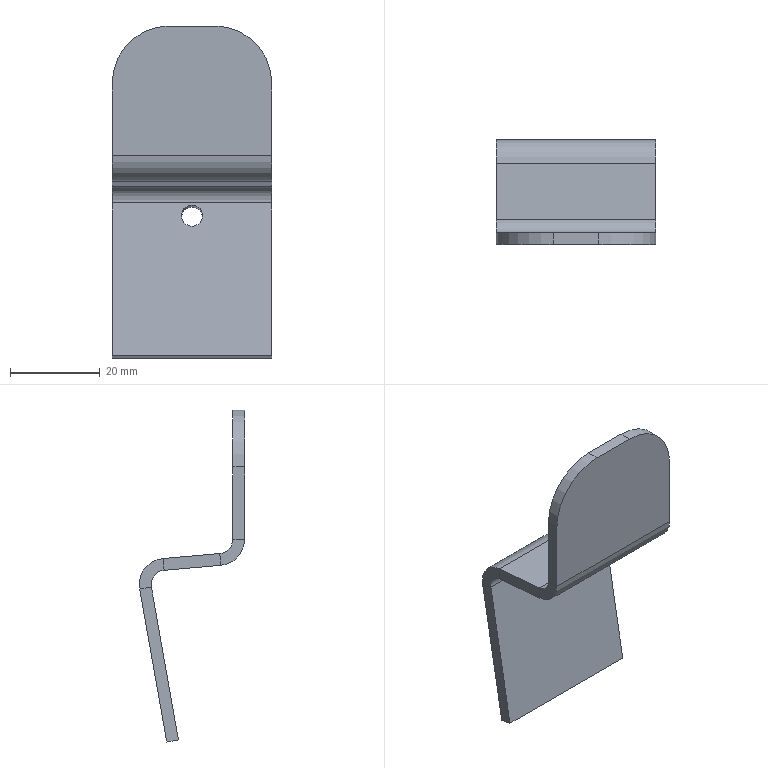Part | NX | features BREP 1 | 1 solid | 26 faces | box 35.56 x 23.477 x 74.022 mm | volume 8250 mm3 | plane 18 | cylinder 8 | commonest cylinder face diameters 4.775 x2 6.35 x2 11.633 x2 25.4 x2
STEP:
#1=CARTESIAN_POINT('',(17.78,0.,-12.7));
#2=VERTEX_POINT('',#1);
#3=CARTESIAN_POINT('',(17.78,0.,-28.841));
#4=VERTEX_POINT('',#3);
#5=CARTESIAN_POINT('',(17.78,0.,-12.7));
#6=DIRECTION('',(0.,0.,-1.));
#7=VECTOR('',#6,1000.);
#8=LINE('',#5,#7);
#9=EDGE_CURVE('',#2,#4,#8,.T.);
#10=ORIENTED_EDGE('',*,*,#9,.T.);
#11=CARTESIAN_POINT('',(-17.78,0.,-28.841));
#12=VERTEX_POINT('',#11);
#13=CARTESIAN_POINT('',(-17.78,0.,-28.841));
#14=DIRECTION('',(1.,0.,0.));
#15=VECTOR('',#14,1000.);
#16=LINE('',#13,#15);
#17=EDGE_CURVE('',#12,#4,#16,.T.);
#18=ORIENTED_EDGE('',*,*,#17,.F.);
#19=CARTESIAN_POINT('',(-17.78,0.,-12.7));
#20=VERTEX_POINT('',#19);
#21=CARTESIAN_POINT('',(-17.78,0.,-28.841));
#22=DIRECTION('',(0.,0.,1.));
#23=VECTOR('',#22,1000.);
#24=LINE('',#21,#23);
#25=EDGE_CURVE('',#12,#20,#24,.T.);
#26=ORIENTED_EDGE('',*,*,#25,.T.);
#27=CARTESIAN_POINT('',(-5.08,0.,0.));
#28=VERTEX_POINT('',#27);
#29=CARTESIAN_POINT('',(-5.08,0.,-12.7));
#30=DIRECTION('',(0.,1.,0.));
#31=DIRECTION('',(-1.,0.,0.));
#32=AXIS2_PLACEMENT_3D('',#29,#30,#31);
#33=CIRCLE('',#32,12.7);
#34=EDGE_CURVE('',#20,#28,#33,.T.);
#35=ORIENTED_EDGE('',*,*,#34,.T.);
#36=CARTESIAN_POINT('',(5.08,0.,0.));
#37=VERTEX_POINT('',#36);
#38=CARTESIAN_POINT('',(-5.08,0.,0.));
#39=DIRECTION('',(1.,0.,0.));
#40=VECTOR('',#39,1000.);
#41=LINE('',#38,#40);
#42=EDGE_CURVE('',#28,#37,#41,.T.);
#43=ORIENTED_EDGE('',*,*,#42,.T.);
#44=CARTESIAN_POINT('',(5.08,0.,-12.7));
#45=DIRECTION('',(0.,1.,0.));
#46=DIRECTION('',(0.,0.,1.));
#47=AXIS2_PLACEMENT_3D('',#44,#45,#46);
#48=CIRCLE('',#47,12.7);
#49=EDGE_CURVE('',#37,#2,#48,.T.);
#50=ORIENTED_EDGE('',*,*,#49,.T.);
#51=EDGE_LOOP('',(#10,#18,#26,#35,#43,#50));
#52=FACE_BOUND('',#51,.T.);
#53=CARTESIAN_POINT('',(0.,0.,0.));
#54=DIRECTION('',(0.,1.,0.));
#55=DIRECTION('',(1.,0.,0.));
#56=AXIS2_PLACEMENT_3D('',#53,#54,#55);
#57=PLANE('',#56);
#58=ADVANCED_FACE('',(#52),#57,.T.);
#59=CARTESIAN_POINT('',(17.78,-2.642,-12.7));
#60=VERTEX_POINT('',#59);
#61=CARTESIAN_POINT('',(5.08,-2.642,0.));
#62=VERTEX_POINT('',#61);
#63=CARTESIAN_POINT('',(5.08,-2.642,-12.7));
#64=DIRECTION('',(0.,-1.,0.));
#65=DIRECTION('',(1.,0.,0.));
#66=AXIS2_PLACEMENT_3D('',#63,#64,#65);
#67=CIRCLE('',#66,12.7);
#68=EDGE_CURVE('',#60,#62,#67,.T.);
#69=ORIENTED_EDGE('',*,*,#68,.F.);
#70=CARTESIAN_POINT('',(17.78,-2.642,-12.7));
#71=DIRECTION('',(0.,1.,0.));
#72=VECTOR('',#71,1000.);
#73=LINE('',#70,#72);
#74=EDGE_CURVE('',#60,#2,#73,.T.);
#75=ORIENTED_EDGE('',*,*,#74,.T.);
#76=ORIENTED_EDGE('',*,*,#49,.F.);
#77=CARTESIAN_POINT('',(5.08,-2.642,0.));
#78=DIRECTION('',(0.,1.,0.));
#79=VECTOR('',#78,1000.);
#80=LINE('',#77,#79);
#81=EDGE_CURVE('',#62,#37,#80,.T.);
#82=ORIENTED_EDGE('',*,*,#81,.F.);
#83=EDGE_LOOP('',(#69,#75,#76,#82));
#84=FACE_BOUND('',#83,.T.);
#85=CARTESIAN_POINT('',(5.08,-2.756,-12.7));
#86=DIRECTION('',(0.,1.,0.));
#87=DIRECTION('',(0.,0.,1.));
#88=AXIS2_PLACEMENT_3D('',#85,#86,#87);
#89=CYLINDRICAL_SURFACE('',#88,12.7);
#90=ADVANCED_FACE('',(#84),#89,.T.);
#91=ORIENTED_EDGE('',*,*,#42,.F.);
#92=CARTESIAN_POINT('',(-5.08,-2.642,0.));
#93=VERTEX_POINT('',#92);
#94=CARTESIAN_POINT('',(-5.08,-2.642,0.));
#95=DIRECTION('',(0.,1.,0.));
#96=VECTOR('',#95,1000.);
#97=LINE('',#94,#96);
#98=EDGE_CURVE('',#93,#28,#97,.T.);
#99=ORIENTED_EDGE('',*,*,#98,.F.);
#100=CARTESIAN_POINT('',(-5.08,-2.642,0.));
#101=DIRECTION('',(1.,0.,0.));
#102=VECTOR('',#101,1000.);
#103=LINE('',#100,#102);
#104=EDGE_CURVE('',#93,#62,#103,.T.);
#105=ORIENTED_EDGE('',*,*,#104,.T.);
#106=ORIENTED_EDGE('',*,*,#81,.T.);
#107=EDGE_LOOP('',(#91,#99,#105,#106));
#108=FACE_BOUND('',#107,.T.);
#109=CARTESIAN_POINT('',(0.,-1.321,0.));
#110=DIRECTION('',(0.,0.,1.));
#111=DIRECTION('',(1.,0.,0.));
#112=AXIS2_PLACEMENT_3D('',#109,#110,#111);
#113=PLANE('',#112);
#114=ADVANCED_FACE('',(#108),#113,.T.);
#115=ORIENTED_EDGE('',*,*,#104,.F.);
#116=CARTESIAN_POINT('',(-17.78,-2.642,-12.7));
#117=VERTEX_POINT('',#116);
#118=CARTESIAN_POINT('',(-5.08,-2.642,-12.7));
#119=DIRECTION('',(0.,-1.,0.));
#120=DIRECTION('',(0.,0.,1.));
#121=AXIS2_PLACEMENT_3D('',#118,#119,#120);
#122=CIRCLE('',#121,12.7);
#123=EDGE_CURVE('',#93,#117,#122,.T.);
#124=ORIENTED_EDGE('',*,*,#123,.T.);
#125=CARTESIAN_POINT('',(-17.78,-2.642,-28.841));
#126=VERTEX_POINT('',#125);
#127=CARTESIAN_POINT('',(-17.78,-2.642,-28.841));
#128=DIRECTION('',(0.,0.,1.));
#129=VECTOR('',#128,1000.);
#130=LINE('',#127,#129);
#131=EDGE_CURVE('',#126,#117,#130,.T.);
#132=ORIENTED_EDGE('',*,*,#131,.F.);
#133=CARTESIAN_POINT('',(17.78,-2.642,-28.841));
#134=VERTEX_POINT('',#133);
#135=CARTESIAN_POINT('',(-17.78,-2.642,-28.841));
#136=DIRECTION('',(1.,0.,0.));
#137=VECTOR('',#136,1000.);
#138=LINE('',#135,#137);
#139=EDGE_CURVE('',#126,#134,#138,.T.);
#140=ORIENTED_EDGE('',*,*,#139,.T.);
#141=CARTESIAN_POINT('',(17.78,-2.642,-12.7));
#142=DIRECTION('',(0.,0.,-1.));
#143=VECTOR('',#142,1000.);
#144=LINE('',#141,#143);
#145=EDGE_CURVE('',#60,#134,#144,.T.);
#146=ORIENTED_EDGE('',*,*,#145,.F.);
#147=ORIENTED_EDGE('',*,*,#68,.T.);
#148=EDGE_LOOP('',(#115,#124,#132,#140,#146,#147));
#149=FACE_BOUND('',#148,.T.);
#150=CARTESIAN_POINT('',(0.,-2.642,0.));
#151=DIRECTION('',(0.,1.,0.));
#152=DIRECTION('',(1.,0.,0.));
#153=AXIS2_PLACEMENT_3D('',#150,#151,#152);
#154=PLANE('',#153);
#155=ADVANCED_FACE('',(#149),#154,.F.);
#156=ORIENTED_EDGE('',*,*,#145,.T.);
#157=CARTESIAN_POINT('',(17.78,0.,-28.841));
#158=DIRECTION('',(0.,-1.,0.));
#159=VECTOR('',#158,1000.);
#160=LINE('',#157,#159);
#161=EDGE_CURVE('',#4,#134,#160,.T.);
#162=ORIENTED_EDGE('',*,*,#161,.F.);
#163=ORIENTED_EDGE('',*,*,#9,.F.);
#164=ORIENTED_EDGE('',*,*,#74,.F.);
#165=EDGE_LOOP('',(#156,#162,#163,#164));
#166=FACE_BOUND('',#165,.T.);
#167=CARTESIAN_POINT('',(17.78,-1.321,-15.875));
#168=DIRECTION('',(1.,0.,0.));
#169=DIRECTION('',(0.,1.,0.));
#170=AXIS2_PLACEMENT_3D('',#167,#168,#169);
#171=PLANE('',#170);
#172=ADVANCED_FACE('',(#166),#171,.T.);
#173=ORIENTED_EDGE('',*,*,#161,.T.);
#174=CARTESIAN_POINT('',(17.78,2.668,-34.635));
#175=VERTEX_POINT('',#174);
#176=CARTESIAN_POINT('',(17.78,3.175,-28.841));
#177=DIRECTION('',(-1.,0.,0.));
#178=DIRECTION('',(0.,-0.08716,-0.9962));
#179=AXIS2_PLACEMENT_3D('',#176,#177,#178);
#180=CIRCLE('',#179,5.817);
#181=EDGE_CURVE('',#175,#134,#180,.T.);
#182=ORIENTED_EDGE('',*,*,#181,.F.);
#183=CARTESIAN_POINT('',(17.78,2.898,-32.004));
#184=VERTEX_POINT('',#183);
#185=CARTESIAN_POINT('',(17.78,2.898,-32.004));
#186=DIRECTION('',(0.,-0.08716,-0.9962));
#187=VECTOR('',#186,1000.);
#188=LINE('',#185,#187);
#189=EDGE_CURVE('',#184,#175,#188,.T.);
#190=ORIENTED_EDGE('',*,*,#189,.F.);
#191=CARTESIAN_POINT('',(17.78,3.175,-28.841));
#192=DIRECTION('',(-1.,0.,0.));
#193=DIRECTION('',(0.,-0.08716,-0.9962));
#194=AXIS2_PLACEMENT_3D('',#191,#192,#193);
#195=CIRCLE('',#194,3.175);
#196=EDGE_CURVE('',#184,#4,#195,.T.);
#197=ORIENTED_EDGE('',*,*,#196,.T.);
#198=EDGE_LOOP('',(#173,#182,#190,#197));
#199=FACE_BOUND('',#198,.T.);
#200=CARTESIAN_POINT('',(17.78,-0.1397,-31.878));
#201=DIRECTION('',(-1.,0.,0.));
#202=DIRECTION('',(0.,0.,1.));
#203=AXIS2_PLACEMENT_3D('',#200,#201,#202);
#204=PLANE('',#203);
#205=ADVANCED_FACE('',(#199),#204,.F.);
#206=CARTESIAN_POINT('',(-17.78,2.898,-32.004));
#207=VERTEX_POINT('',#206);
#208=CARTESIAN_POINT('',(-17.78,3.175,-28.841));
#209=DIRECTION('',(-1.,0.,0.));
#210=DIRECTION('',(0.,-0.08716,-0.9962));
#211=AXIS2_PLACEMENT_3D('',#208,#209,#210);
#212=CIRCLE('',#211,3.175);
#213=EDGE_CURVE('',#207,#12,#212,.T.);
#214=ORIENTED_EDGE('',*,*,#213,.T.);
#215=ORIENTED_EDGE('',*,*,#17,.T.);
#216=ORIENTED_EDGE('',*,*,#196,.F.);
#217=CARTESIAN_POINT('',(-17.78,2.898,-32.004));
#218=DIRECTION('',(1.,0.,0.));
#219=VECTOR('',#218,1000.);
#220=LINE('',#217,#219);
#221=EDGE_CURVE('',#207,#184,#220,.T.);
#222=ORIENTED_EDGE('',*,*,#221,.F.);
#223=EDGE_LOOP('',(#214,#215,#216,#222));
#224=FACE_BOUND('',#223,.T.);
#225=CARTESIAN_POINT('',(-17.78,3.175,-28.841));
#226=DIRECTION('',(-1.,0.,0.));
#227=DIRECTION('',(0.,-0.08716,-0.9962));
#228=AXIS2_PLACEMENT_3D('',#225,#226,#227);
#229=CYLINDRICAL_SURFACE('',#228,3.175);
#230=ADVANCED_FACE('',(#224),#229,.F.);
#231=CARTESIAN_POINT('',(17.78,15.526,-33.108));
#232=VERTEX_POINT('',#231);
#233=CARTESIAN_POINT('',(-17.78,15.526,-33.108));
#234=VERTEX_POINT('',#233);
#235=CARTESIAN_POINT('',(17.78,15.526,-33.108));
#236=DIRECTION('',(-1.,0.,0.));
#237=VECTOR('',#236,1000.);
#238=LINE('',#235,#237);
#239=EDGE_CURVE('',#232,#234,#238,.T.);
#240=ORIENTED_EDGE('',*,*,#239,.T.);
#241=CARTESIAN_POINT('',(-17.78,15.526,-33.108));
#242=DIRECTION('',(0.,-0.9962,0.08716));
#243=VECTOR('',#242,1000.);
#244=LINE('',#241,#243);
#245=EDGE_CURVE('',#234,#207,#244,.T.);
#246=ORIENTED_EDGE('',*,*,#245,.T.);
#247=ORIENTED_EDGE('',*,*,#221,.T.);
#248=CARTESIAN_POINT('',(17.78,2.898,-32.004));
#249=DIRECTION('',(0.,0.9962,-0.08716));
#250=VECTOR('',#249,1000.);
#251=LINE('',#248,#250);
#252=EDGE_CURVE('',#184,#232,#251,.T.);
#253=ORIENTED_EDGE('',*,*,#252,.T.);
#254=EDGE_LOOP('',(#240,#246,#247,#253));
#255=FACE_BOUND('',#254,.T.);
#256=CARTESIAN_POINT('',(9.331,0.,-31.75));
#257=DIRECTION('',(0.,0.08716,0.9962));
#258=DIRECTION('',(1.,0.,0.));
#259=AXIS2_PLACEMENT_3D('',#256,#257,#258);
#260=PLANE('',#259);
#261=ADVANCED_FACE('',(#255),#260,.T.);
#262=ORIENTED_EDGE('',*,*,#189,.T.);
#263=CARTESIAN_POINT('',(17.78,15.296,-35.74));
#264=VERTEX_POINT('',#263);
#265=CARTESIAN_POINT('',(17.78,2.668,-34.635));
#266=DIRECTION('',(0.,0.9962,-0.08716));
#267=VECTOR('',#266,1000.);
#268=LINE('',#265,#267);
#269=EDGE_CURVE('',#175,#264,#268,.T.);
#270=ORIENTED_EDGE('',*,*,#269,.T.);
#271=CARTESIAN_POINT('',(17.78,15.296,-35.74));
#272=DIRECTION('',(0.,0.08716,0.9962));
#273=VECTOR('',#272,1000.);
#274=LINE('',#271,#273);
#275=EDGE_CURVE('',#264,#232,#274,.T.);
#276=ORIENTED_EDGE('',*,*,#275,.T.);
#277=ORIENTED_EDGE('',*,*,#252,.F.);
#278=EDGE_LOOP('',(#262,#270,#276,#277));
#279=FACE_BOUND('',#278,.T.);
#280=CARTESIAN_POINT('',(17.78,10.823,-34.023));
#281=DIRECTION('',(1.,0.,0.));
#282=DIRECTION('',(0.,1.,0.));
#283=AXIS2_PLACEMENT_3D('',#280,#281,#282);
#284=PLANE('',#283);
#285=ADVANCED_FACE('',(#279),#284,.T.);
#286=CARTESIAN_POINT('',(17.78,18.146,-39.454));
#287=VERTEX_POINT('',#286);
#288=CARTESIAN_POINT('',(17.78,20.747,-39.913));
#289=VERTEX_POINT('',#288);
#290=CARTESIAN_POINT('',(17.78,18.146,-39.454));
#291=DIRECTION('',(0.,0.9848,-0.1736));
#292=VECTOR('',#291,1000.);
#293=LINE('',#290,#292);
#294=EDGE_CURVE('',#287,#289,#293,.T.);
#295=ORIENTED_EDGE('',*,*,#294,.T.);
#296=CARTESIAN_POINT('',(17.78,15.019,-38.903));
#297=DIRECTION('',(1.,0.,0.));
#298=DIRECTION('',(0.,0.9848,-0.1736));
#299=AXIS2_PLACEMENT_3D('',#296,#297,#298);
#300=CIRCLE('',#299,5.817);
#301=EDGE_CURVE('',#289,#232,#300,.T.);
#302=ORIENTED_EDGE('',*,*,#301,.T.);
#303=ORIENTED_EDGE('',*,*,#275,.F.);
#304=CARTESIAN_POINT('',(17.78,15.019,-38.903));
#305=DIRECTION('',(1.,0.,0.));
#306=DIRECTION('',(0.,0.9848,-0.1736));
#307=AXIS2_PLACEMENT_3D('',#304,#305,#306);
#308=CIRCLE('',#307,3.175);
#309=EDGE_CURVE('',#287,#264,#308,.T.);
#310=ORIENTED_EDGE('',*,*,#309,.F.);
#311=EDGE_LOOP('',(#295,#302,#303,#310));
#312=FACE_BOUND('',#311,.T.);
#313=CARTESIAN_POINT('',(17.78,18.586,-36.166));
#314=DIRECTION('',(1.,0.,0.));
#315=DIRECTION('',(0.,1.,0.));
#316=AXIS2_PLACEMENT_3D('',#313,#314,#315);
#317=PLANE('',#316);
#318=ADVANCED_FACE('',(#312),#317,.T.);
#319=ORIENTED_EDGE('',*,*,#309,.T.);
#320=CARTESIAN_POINT('',(-17.78,15.296,-35.74));
#321=VERTEX_POINT('',#320);
#322=CARTESIAN_POINT('',(17.78,15.296,-35.74));
#323=DIRECTION('',(-1.,0.,0.));
#324=VECTOR('',#323,1000.);
#325=LINE('',#322,#324);
#326=EDGE_CURVE('',#264,#321,#325,.T.);
#327=ORIENTED_EDGE('',*,*,#326,.T.);
#328=CARTESIAN_POINT('',(-17.78,18.146,-39.454));
#329=VERTEX_POINT('',#328);
#330=CARTESIAN_POINT('',(-17.78,15.019,-38.903));
#331=DIRECTION('',(1.,0.,0.));
#332=DIRECTION('',(0.,0.9848,-0.1736));
#333=AXIS2_PLACEMENT_3D('',#330,#331,#332);
#334=CIRCLE('',#333,3.175);
#335=EDGE_CURVE('',#329,#321,#334,.T.);
#336=ORIENTED_EDGE('',*,*,#335,.F.);
#337=CARTESIAN_POINT('',(17.78,18.146,-39.454));
#338=DIRECTION('',(-1.,0.,0.));
#339=VECTOR('',#338,1000.);
#340=LINE('',#337,#339);
#341=EDGE_CURVE('',#287,#329,#340,.T.);
#342=ORIENTED_EDGE('',*,*,#341,.F.);
#343=EDGE_LOOP('',(#319,#327,#336,#342));
#344=FACE_BOUND('',#343,.T.);
#345=CARTESIAN_POINT('',(17.78,15.019,-38.903));
#346=DIRECTION('',(1.,0.,0.));
#347=DIRECTION('',(0.,0.9848,-0.1736));
#348=AXIS2_PLACEMENT_3D('',#345,#346,#347);
#349=CYLINDRICAL_SURFACE('',#348,3.175);
#350=ADVANCED_FACE('',(#344),#349,.F.);
#351=CARTESIAN_POINT('',(-17.78,12.131,-73.563));
#352=VERTEX_POINT('',#351);
#353=CARTESIAN_POINT('',(17.78,12.131,-73.563));
#354=VERTEX_POINT('',#353);
#355=CARTESIAN_POINT('',(-17.78,12.131,-73.563));
#356=DIRECTION('',(1.,0.,0.));
#357=VECTOR('',#356,1000.);
#358=LINE('',#355,#357);
#359=EDGE_CURVE('',#352,#354,#358,.T.);
#360=ORIENTED_EDGE('',*,*,#359,.T.);
#361=CARTESIAN_POINT('',(17.78,12.131,-73.563));
#362=DIRECTION('',(0.,0.1736,0.9848));
#363=VECTOR('',#362,1000.);
#364=LINE('',#361,#363);
#365=EDGE_CURVE('',#354,#287,#364,.T.);
#366=ORIENTED_EDGE('',*,*,#365,.T.);
#367=ORIENTED_EDGE('',*,*,#341,.T.);
#368=CARTESIAN_POINT('',(-17.78,18.146,-39.454));
#369=DIRECTION('',(0.,-0.1736,-0.9848));
#370=VECTOR('',#369,1000.);
#371=LINE('',#368,#370);
#372=EDGE_CURVE('',#329,#352,#371,.T.);
#373=ORIENTED_EDGE('',*,*,#372,.T.);
#374=EDGE_LOOP('',(#360,#366,#367,#373));
#375=FACE_BOUND('',#374,.T.);
#376=CARTESIAN_POINT('',(2.388,17.645,-42.295));
#377=VERTEX_POINT('',#376);
#378=CARTESIAN_POINT('',(-2.388,17.645,-42.295));
#379=VERTEX_POINT('',#378);
#380=CARTESIAN_POINT('',(0.,17.645,-42.295));
#381=DIRECTION('',(0.,0.9848,-0.1736));
#382=DIRECTION('',(1.,0.,0.));
#383=AXIS2_PLACEMENT_3D('',#380,#381,#382);
#384=CIRCLE('',#383,2.388);
#385=EDGE_CURVE('',#377,#379,#384,.T.);
#386=ORIENTED_EDGE('',*,*,#385,.T.);
#387=CARTESIAN_POINT('',(0.,17.645,-42.295));
#388=DIRECTION('',(0.,0.9848,-0.1736));
#389=DIRECTION('',(-1.,0.,0.));
#390=AXIS2_PLACEMENT_3D('',#387,#388,#389);
#391=CIRCLE('',#390,2.388);
#392=EDGE_CURVE('',#379,#377,#391,.T.);
#393=ORIENTED_EDGE('',*,*,#392,.T.);
#394=EDGE_LOOP('',(#386,#393));
#395=FACE_BOUND('',#394,.T.);
#396=CARTESIAN_POINT('',(9.331,18.747,-36.042));
#397=DIRECTION('',(0.,-0.9848,0.1736));
#398=DIRECTION('',(-1.,0.,0.));
#399=AXIS2_PLACEMENT_3D('',#396,#397,#398);
#400=PLANE('',#399);
#401=ADVANCED_FACE('',(#375,#395),#400,.T.);
#402=CARTESIAN_POINT('',(-17.78,20.747,-39.913));
#403=VERTEX_POINT('',#402);
#404=CARTESIAN_POINT('',(-17.78,18.146,-39.454));
#405=DIRECTION('',(0.,0.9848,-0.1736));
#406=VECTOR('',#405,1000.);
#407=LINE('',#404,#406);
#408=EDGE_CURVE('',#329,#403,#407,.T.);
#409=ORIENTED_EDGE('',*,*,#408,.T.);
#410=CARTESIAN_POINT('',(-17.78,14.733,-74.022));
#411=VERTEX_POINT('',#410);
#412=CARTESIAN_POINT('',(-17.78,20.747,-39.913));
#413=DIRECTION('',(0.,-0.1736,-0.9848));
#414=VECTOR('',#413,1000.);
#415=LINE('',#412,#414);
#416=EDGE_CURVE('',#403,#411,#415,.T.);
#417=ORIENTED_EDGE('',*,*,#416,.T.);
#418=CARTESIAN_POINT('',(-17.78,12.131,-73.563));
#419=DIRECTION('',(0.,0.9848,-0.1736));
#420=VECTOR('',#419,1000.);
#421=LINE('',#418,#420);
#422=EDGE_CURVE('',#352,#411,#421,.T.);
#423=ORIENTED_EDGE('',*,*,#422,.F.);
#424=ORIENTED_EDGE('',*,*,#372,.F.);
#425=EDGE_LOOP('',(#409,#417,#423,#424));
#426=FACE_BOUND('',#425,.T.);
#427=CARTESIAN_POINT('',(-17.78,16.439,-56.738));
#428=DIRECTION('',(-1.,0.,0.));
#429=DIRECTION('',(0.,0.,1.));
#430=AXIS2_PLACEMENT_3D('',#427,#428,#429);
#431=PLANE('',#430);
#432=ADVANCED_FACE('',(#426),#431,.T.);
#433=ORIENTED_EDGE('',*,*,#422,.T.);
#434=CARTESIAN_POINT('',(17.78,14.733,-74.022));
#435=VERTEX_POINT('',#434);
#436=CARTESIAN_POINT('',(-17.78,14.733,-74.022));
#437=DIRECTION('',(1.,0.,0.));
#438=VECTOR('',#437,1000.);
#439=LINE('',#436,#438);
#440=EDGE_CURVE('',#411,#435,#439,.T.);
#441=ORIENTED_EDGE('',*,*,#440,.T.);
#442=CARTESIAN_POINT('',(17.78,12.131,-73.563));
#443=DIRECTION('',(0.,0.9848,-0.1736));
#444=VECTOR('',#443,1000.);
#445=LINE('',#442,#444);
#446=EDGE_CURVE('',#354,#435,#445,.T.);
#447=ORIENTED_EDGE('',*,*,#446,.F.);
#448=ORIENTED_EDGE('',*,*,#359,.F.);
#449=EDGE_LOOP('',(#433,#441,#447,#448));
#450=FACE_BOUND('',#449,.T.);
#451=CARTESIAN_POINT('',(0.,13.432,-73.792));
#452=DIRECTION('',(0.,-0.1736,-0.9848));
#453=DIRECTION('',(0.,-0.9848,0.1736));
#454=AXIS2_PLACEMENT_3D('',#451,#452,#453);
#455=PLANE('',#454);
#456=ADVANCED_FACE('',(#450),#455,.T.);
#457=ORIENTED_EDGE('',*,*,#446,.T.);
#458=CARTESIAN_POINT('',(17.78,14.733,-74.022));
#459=DIRECTION('',(0.,0.1736,0.9848));
#460=VECTOR('',#459,1000.);
#461=LINE('',#458,#460);
#462=EDGE_CURVE('',#435,#289,#461,.T.);
#463=ORIENTED_EDGE('',*,*,#462,.T.);
#464=ORIENTED_EDGE('',*,*,#294,.F.);
#465=ORIENTED_EDGE('',*,*,#365,.F.);
#466=EDGE_LOOP('',(#457,#463,#464,#465));
#467=FACE_BOUND('',#466,.T.);
#468=CARTESIAN_POINT('',(17.78,16.439,-56.738));
#469=DIRECTION('',(1.,0.,0.));
#470=DIRECTION('',(0.,1.,0.));
#471=AXIS2_PLACEMENT_3D('',#468,#469,#470);
#472=PLANE('',#471);
#473=ADVANCED_FACE('',(#467),#472,.T.);
#474=CARTESIAN_POINT('',(17.78,20.747,-39.913));
#475=DIRECTION('',(-1.,0.,0.));
#476=VECTOR('',#475,1000.);
#477=LINE('',#474,#476);
#478=EDGE_CURVE('',#289,#403,#477,.T.);
#479=ORIENTED_EDGE('',*,*,#478,.F.);
#480=ORIENTED_EDGE('',*,*,#462,.F.);
#481=ORIENTED_EDGE('',*,*,#440,.F.);
#482=ORIENTED_EDGE('',*,*,#416,.F.);
#483=EDGE_LOOP('',(#479,#480,#481,#482));
#484=FACE_BOUND('',#483,.T.);
#485=CARTESIAN_POINT('',(2.388,20.246,-42.754));
#486=VERTEX_POINT('',#485);
#487=CARTESIAN_POINT('',(-2.388,20.246,-42.754));
#488=VERTEX_POINT('',#487);
#489=CARTESIAN_POINT('',(0.,20.246,-42.754));
#490=DIRECTION('',(0.,0.9848,-0.1736));
#491=DIRECTION('',(1.,0.,0.));
#492=AXIS2_PLACEMENT_3D('',#489,#490,#491);
#493=CIRCLE('',#492,2.388);
#494=EDGE_CURVE('',#486,#488,#493,.T.);
#495=ORIENTED_EDGE('',*,*,#494,.F.);
#496=CARTESIAN_POINT('',(0.,20.246,-42.754));
#497=DIRECTION('',(0.,0.9848,-0.1736));
#498=DIRECTION('',(-1.,0.,0.));
#499=AXIS2_PLACEMENT_3D('',#496,#497,#498);
#500=CIRCLE('',#499,2.388);
#501=EDGE_CURVE('',#488,#486,#500,.T.);
#502=ORIENTED_EDGE('',*,*,#501,.F.);
#503=EDGE_LOOP('',(#495,#502));
#504=FACE_BOUND('',#503,.T.);
#505=CARTESIAN_POINT('',(9.331,21.349,-36.501));
#506=DIRECTION('',(0.,-0.9848,0.1736));
#507=DIRECTION('',(-1.,0.,0.));
#508=AXIS2_PLACEMENT_3D('',#505,#506,#507);
#509=PLANE('',#508);
#510=ADVANCED_FACE('',(#484,#504),#509,.F.);
#511=CARTESIAN_POINT('',(-17.78,15.019,-38.903));
#512=DIRECTION('',(1.,0.,0.));
#513=DIRECTION('',(0.,0.9848,-0.1736));
#514=AXIS2_PLACEMENT_3D('',#511,#512,#513);
#515=CIRCLE('',#514,5.817);
#516=EDGE_CURVE('',#403,#234,#515,.T.);
#517=ORIENTED_EDGE('',*,*,#516,.T.);
#518=ORIENTED_EDGE('',*,*,#239,.F.);
#519=ORIENTED_EDGE('',*,*,#301,.F.);
#520=ORIENTED_EDGE('',*,*,#478,.T.);
#521=EDGE_LOOP('',(#517,#518,#519,#520));
#522=FACE_BOUND('',#521,.T.);
#523=CARTESIAN_POINT('',(17.78,15.019,-38.903));
#524=DIRECTION('',(1.,0.,0.));
#525=DIRECTION('',(0.,0.9848,-0.1736));
#526=AXIS2_PLACEMENT_3D('',#523,#524,#525);
#527=CYLINDRICAL_SURFACE('',#526,5.817);
#528=ADVANCED_FACE('',(#522),#527,.T.);
#529=CARTESIAN_POINT('',(-17.78,15.296,-35.74));
#530=DIRECTION('',(0.,0.08716,0.9962));
#531=VECTOR('',#530,1000.);
#532=LINE('',#529,#531);
#533=EDGE_CURVE('',#321,#234,#532,.T.);
#534=ORIENTED_EDGE('',*,*,#533,.T.);
#535=ORIENTED_EDGE('',*,*,#516,.F.);
#536=ORIENTED_EDGE('',*,*,#408,.F.);
#537=ORIENTED_EDGE('',*,*,#335,.T.);
#538=EDGE_LOOP('',(#534,#535,#536,#537));
#539=FACE_BOUND('',#538,.T.);
#540=CARTESIAN_POINT('',(-17.78,18.586,-36.166));
#541=DIRECTION('',(1.,0.,0.));
#542=DIRECTION('',(0.,1.,0.));
#543=AXIS2_PLACEMENT_3D('',#540,#541,#542);
#544=PLANE('',#543);
#545=ADVANCED_FACE('',(#539),#544,.F.);
#546=ORIENTED_EDGE('',*,*,#533,.F.);
#547=CARTESIAN_POINT('',(-17.78,2.668,-34.635));
#548=VERTEX_POINT('',#547);
#549=CARTESIAN_POINT('',(-17.78,15.296,-35.74));
#550=DIRECTION('',(0.,-0.9962,0.08716));
#551=VECTOR('',#550,1000.);
#552=LINE('',#549,#551);
#553=EDGE_CURVE('',#321,#548,#552,.T.);
#554=ORIENTED_EDGE('',*,*,#553,.T.);
#555=CARTESIAN_POINT('',(-17.78,2.898,-32.004));
#556=DIRECTION('',(0.,-0.08716,-0.9962));
#557=VECTOR('',#556,1000.);
#558=LINE('',#555,#557);
#559=EDGE_CURVE('',#207,#548,#558,.T.);
#560=ORIENTED_EDGE('',*,*,#559,.F.);
#561=ORIENTED_EDGE('',*,*,#245,.F.);
#562=EDGE_LOOP('',(#546,#554,#560,#561));
#563=FACE_BOUND('',#562,.T.);
#564=CARTESIAN_POINT('',(-17.78,10.823,-34.023));
#565=DIRECTION('',(-1.,0.,0.));
#566=DIRECTION('',(0.,0.,1.));
#567=AXIS2_PLACEMENT_3D('',#564,#565,#566);
#568=PLANE('',#567);
#569=ADVANCED_FACE('',(#563),#568,.T.);
#570=ORIENTED_EDGE('',*,*,#559,.T.);
#571=CARTESIAN_POINT('',(-17.78,3.175,-28.841));
#572=DIRECTION('',(-1.,0.,0.));
#573=DIRECTION('',(0.,-0.08716,-0.9962));
#574=AXIS2_PLACEMENT_3D('',#571,#572,#573);
#575=CIRCLE('',#574,5.817);
#576=EDGE_CURVE('',#548,#126,#575,.T.);
#577=ORIENTED_EDGE('',*,*,#576,.T.);
#578=CARTESIAN_POINT('',(-17.78,0.,-28.841));
#579=DIRECTION('',(0.,-1.,0.));
#580=VECTOR('',#579,1000.);
#581=LINE('',#578,#580);
#582=EDGE_CURVE('',#12,#126,#581,.T.);
#583=ORIENTED_EDGE('',*,*,#582,.F.);
#584=ORIENTED_EDGE('',*,*,#213,.F.);
#585=EDGE_LOOP('',(#570,#577,#583,#584));
#586=FACE_BOUND('',#585,.T.);
#587=CARTESIAN_POINT('',(-17.78,-0.1397,-31.878));
#588=DIRECTION('',(-1.,0.,0.));
#589=DIRECTION('',(0.,0.,1.));
#590=AXIS2_PLACEMENT_3D('',#587,#588,#589);
#591=PLANE('',#590);
#592=ADVANCED_FACE('',(#586),#591,.T.);
#593=ORIENTED_EDGE('',*,*,#25,.F.);
#594=ORIENTED_EDGE('',*,*,#582,.T.);
#595=ORIENTED_EDGE('',*,*,#131,.T.);
#596=CARTESIAN_POINT('',(-17.78,-2.642,-12.7));
#597=DIRECTION('',(0.,1.,0.));
#598=VECTOR('',#597,1000.);
#599=LINE('',#596,#598);
#600=EDGE_CURVE('',#117,#20,#599,.T.);
#601=ORIENTED_EDGE('',*,*,#600,.T.);
#602=EDGE_LOOP('',(#593,#594,#595,#601));
#603=FACE_BOUND('',#602,.T.);
#604=CARTESIAN_POINT('',(-17.78,-1.321,-15.875));
#605=DIRECTION('',(-1.,0.,0.));
#606=DIRECTION('',(0.,0.,1.));
#607=AXIS2_PLACEMENT_3D('',#604,#605,#606);
#608=PLANE('',#607);
#609=ADVANCED_FACE('',(#603),#608,.T.);
#610=ORIENTED_EDGE('',*,*,#123,.F.);
#611=ORIENTED_EDGE('',*,*,#98,.T.);
#612=ORIENTED_EDGE('',*,*,#34,.F.);
#613=ORIENTED_EDGE('',*,*,#600,.F.);
#614=EDGE_LOOP('',(#610,#611,#612,#613));
#615=FACE_BOUND('',#614,.T.);
#616=CARTESIAN_POINT('',(-5.08,-2.756,-12.7));
#617=DIRECTION('',(0.,1.,0.));
#618=DIRECTION('',(-1.,0.,0.));
#619=AXIS2_PLACEMENT_3D('',#616,#617,#618);
#620=CYLINDRICAL_SURFACE('',#619,12.7);
#621=ADVANCED_FACE('',(#615),#620,.T.);
#622=ORIENTED_EDGE('',*,*,#181,.T.);
#623=ORIENTED_EDGE('',*,*,#139,.F.);
#624=ORIENTED_EDGE('',*,*,#576,.F.);
#625=CARTESIAN_POINT('',(-17.78,2.668,-34.635));
#626=DIRECTION('',(1.,0.,0.));
#627=VECTOR('',#626,1000.);
#628=LINE('',#625,#627);
#629=EDGE_CURVE('',#548,#175,#628,.T.);
#630=ORIENTED_EDGE('',*,*,#629,.T.);
#631=EDGE_LOOP('',(#622,#623,#624,#630));
#632=FACE_BOUND('',#631,.T.);
#633=CARTESIAN_POINT('',(-17.78,3.175,-28.841));
#634=DIRECTION('',(-1.,0.,0.));
#635=DIRECTION('',(0.,-0.08716,-0.9962));
#636=AXIS2_PLACEMENT_3D('',#633,#634,#635);
#637=CYLINDRICAL_SURFACE('',#636,5.817);
#638=ADVANCED_FACE('',(#632),#637,.T.);
#639=ORIENTED_EDGE('',*,*,#629,.F.);
#640=ORIENTED_EDGE('',*,*,#553,.F.);
#641=ORIENTED_EDGE('',*,*,#326,.F.);
#642=ORIENTED_EDGE('',*,*,#269,.F.);
#643=EDGE_LOOP('',(#639,#640,#641,#642));
#644=FACE_BOUND('',#643,.T.);
#645=CARTESIAN_POINT('',(9.331,-0.2302,-34.382));
#646=DIRECTION('',(0.,0.08716,0.9962));
#647=DIRECTION('',(1.,0.,0.));
#648=AXIS2_PLACEMENT_3D('',#645,#646,#647);
#649=PLANE('',#648);
#650=ADVANCED_FACE('',(#644),#649,.F.);
#651=CARTESIAN_POINT('',(2.388,20.246,-42.754));
#652=DIRECTION('',(0.,-0.9848,0.1736));
#653=VECTOR('',#652,1000.);
#654=LINE('',#651,#653);
#655=EDGE_CURVE('',#377,#486,#654,.F.);
#656=ORIENTED_EDGE('',*,*,#655,.F.);
#657=ORIENTED_EDGE('',*,*,#392,.F.);
#658=CARTESIAN_POINT('',(-2.388,20.246,-42.754));
#659=DIRECTION('',(0.,-0.9848,0.1736));
#660=VECTOR('',#659,1000.);
#661=LINE('',#658,#660);
#662=EDGE_CURVE('',#379,#488,#661,.F.);
#663=ORIENTED_EDGE('',*,*,#662,.T.);
#664=ORIENTED_EDGE('',*,*,#501,.T.);
#665=EDGE_LOOP('',(#656,#657,#663,#664));
#666=FACE_BOUND('',#665,.T.);
#667=CARTESIAN_POINT('',(0.,18.945,-42.525));
#668=DIRECTION('',(0.,0.9848,-0.1736));
#669=DIRECTION('',(-1.,0.,0.));
#670=AXIS2_PLACEMENT_3D('',#667,#668,#669);
#671=CYLINDRICAL_SURFACE('',#670,2.388);
#672=ADVANCED_FACE('',(#666),#671,.F.);
#673=ORIENTED_EDGE('',*,*,#662,.F.);
#674=ORIENTED_EDGE('',*,*,#385,.F.);
#675=ORIENTED_EDGE('',*,*,#655,.T.);
#676=ORIENTED_EDGE('',*,*,#494,.T.);
#677=EDGE_LOOP('',(#673,#674,#675,#676));
#678=FACE_BOUND('',#677,.T.);
#679=CARTESIAN_POINT('',(0.,18.945,-42.525));
#680=DIRECTION('',(0.,0.9848,-0.1736));
#681=DIRECTION('',(1.,0.,0.));
#682=AXIS2_PLACEMENT_3D('',#679,#680,#681);
#683=CYLINDRICAL_SURFACE('',#682,2.388);
#684=ADVANCED_FACE('',(#678),#683,.F.);
#685=CLOSED_SHELL('',(#58,#90,#114,#155,#172,#205,#230,#261,#285,#318,#350,#401,#432,#456,#473,#510,#528,#545,#569,#592,#609,#621,#638,#650,#672,#684));
#686=MANIFOLD_SOLID_BREP('',#685);
#687=(LENGTH_UNIT()NAMED_UNIT(*)SI_UNIT(.MILLI.,.METRE.));
#688=UNCERTAINTY_MEASURE_WITH_UNIT(LENGTH_MEASURE(0.00001),#687,'','');
#689=(NAMED_UNIT(*)PLANE_ANGLE_UNIT()SI_UNIT($,.RADIAN.));
#690=(NAMED_UNIT(*)SI_UNIT($,.STERADIAN.)SOLID_ANGLE_UNIT());
#691=(GEOMETRIC_REPRESENTATION_CONTEXT(3)GLOBAL_UNCERTAINTY_ASSIGNED_CONTEXT((#688))GLOBAL_UNIT_ASSIGNED_CONTEXT((#687,#689,#690))REPRESENTATION_CONTEXT('',''));
#692=ADVANCED_BREP_SHAPE_REPRESENTATION('',(#686),#691);